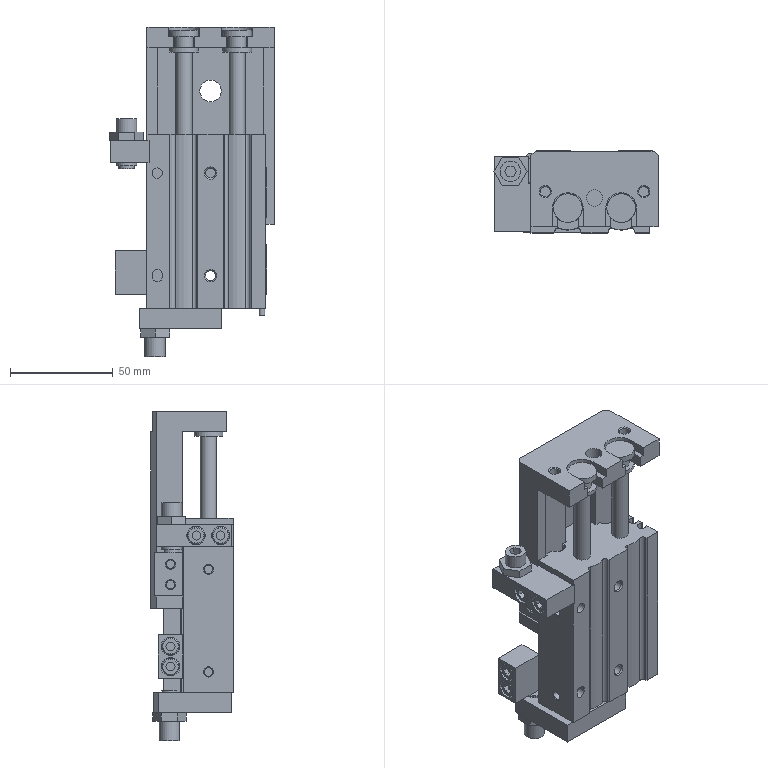Part | NX | 7 solids | 405 faces | box 80.083 x 40 x 160.5 mm | volume 216299 mm3 | plane 279 | cylinder 99 | cone 26 | spline 1 | commonest cylinder face diameters 4.134 x14 9 x10 8.5 x8 10 x8 4 x6 5 x6